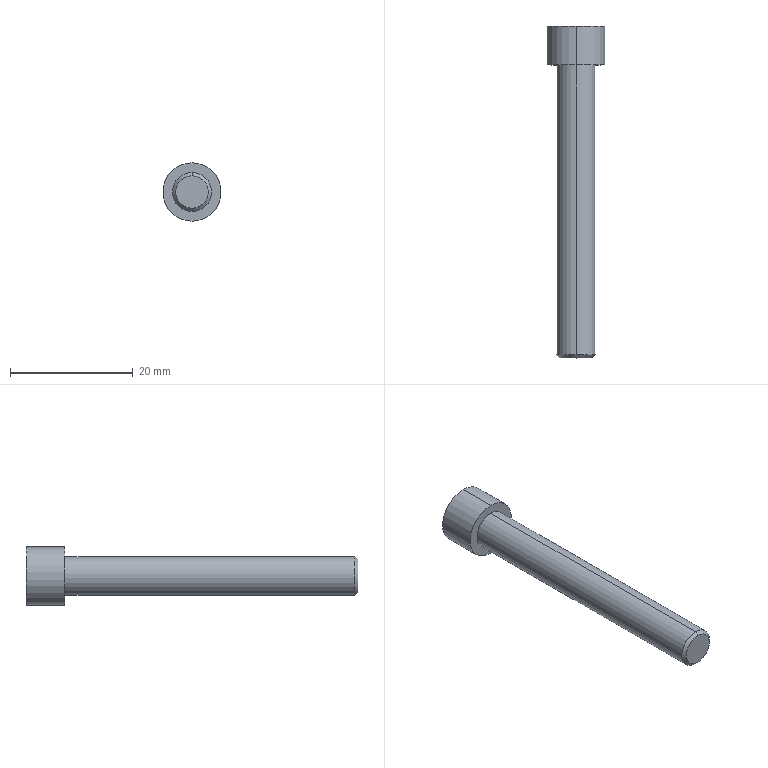Part | STEP file | 4-20.sldasm-Part-206 | 1 solid | 16 faces | box 9.525 x 54.15 x 9.525 mm | volume 1881 mm3 | plane 10 | cylinder 4 | cone 2 | commonest cylinder face diameters 6.35 x2 9.525 x2
STEP:
#1=CARTESIAN_POINT('',(270.795,526.888,-90.641));
#2=VERTEX_POINT('',#1);
#3=CARTESIAN_POINT('',(270.795,526.888,-95.959));
#4=VERTEX_POINT('',#3);
#5=CARTESIAN_POINT('',(270.795,526.888,-93.3));
#6=DIRECTION('',(0.,1.,0.));
#7=DIRECTION('',(0.,0.,1.));
#8=AXIS2_PLACEMENT_3D('',#5,#6,#7);
#9=CIRCLE('',#8,2.659);
#10=EDGE_CURVE('',#2,#4,#9,.T.);
#11=ORIENTED_EDGE('',*,*,#10,.T.);
#12=CARTESIAN_POINT('',(270.795,527.404,-96.475));
#13=VERTEX_POINT('',#12);
#14=CARTESIAN_POINT('',(270.795,527.404,-96.475));
#15=DIRECTION('',(0.,0.7071,-0.7071));
#16=VECTOR('',#15,1000.);
#17=LINE('',#14,#16);
#18=EDGE_CURVE('',#4,#13,#17,.T.);
#19=ORIENTED_EDGE('',*,*,#18,.T.);
#20=CARTESIAN_POINT('',(270.795,527.404,-90.125));
#21=VERTEX_POINT('',#20);
#22=CARTESIAN_POINT('',(270.795,527.404,-93.3));
#23=DIRECTION('',(0.,-1.,0.));
#24=DIRECTION('',(0.,0.,1.));
#25=AXIS2_PLACEMENT_3D('',#22,#23,#24);
#26=CIRCLE('',#25,3.175);
#27=EDGE_CURVE('',#13,#21,#26,.T.);
#28=ORIENTED_EDGE('',*,*,#27,.T.);
#29=CARTESIAN_POINT('',(270.795,527.404,-90.125));
#30=DIRECTION('',(0.,0.7071,0.7071));
#31=VECTOR('',#30,1000.);
#32=LINE('',#29,#31);
#33=EDGE_CURVE('',#2,#21,#32,.T.);
#34=ORIENTED_EDGE('',*,*,#33,.F.);
#35=EDGE_LOOP('',(#11,#19,#28,#34));
#36=FACE_OUTER_BOUND('',#35,.T.);
#37=CARTESIAN_POINT('',(270.795,527.404,-93.3));
#38=DIRECTION('',(0.,1.,0.));
#39=DIRECTION('',(0.,0.,1.));
#40=AXIS2_PLACEMENT_3D('',#37,#38,#39);
#41=CONICAL_SURFACE('',#40,3.175,0.7854);
#42=ADVANCED_FACE('',(#36),#41,.T.);
#43=CARTESIAN_POINT('',(270.795,574.688,-98.063));
#44=VERTEX_POINT('',#43);
#45=CARTESIAN_POINT('',(270.795,574.688,-88.538));
#46=VERTEX_POINT('',#45);
#47=CARTESIAN_POINT('',(270.795,574.688,-93.3));
#48=DIRECTION('',(0.,-1.,0.));
#49=DIRECTION('',(0.,0.,1.));
#50=AXIS2_PLACEMENT_3D('',#47,#48,#49);
#51=CIRCLE('',#50,4.763);
#52=EDGE_CURVE('',#44,#46,#51,.T.);
#53=ORIENTED_EDGE('',*,*,#52,.F.);
#54=CARTESIAN_POINT('',(270.795,581.038,-98.063));
#55=VERTEX_POINT('',#54);
#56=CARTESIAN_POINT('',(270.795,574.688,-98.063));
#57=DIRECTION('',(0.,1.,0.));
#58=VECTOR('',#57,1000.);
#59=LINE('',#56,#58);
#60=EDGE_CURVE('',#44,#55,#59,.T.);
#61=ORIENTED_EDGE('',*,*,#60,.T.);
#62=CARTESIAN_POINT('',(270.795,581.038,-88.538));
#63=VERTEX_POINT('',#62);
#64=CARTESIAN_POINT('',(270.795,581.038,-93.3));
#65=DIRECTION('',(0.,-1.,0.));
#66=DIRECTION('',(0.,0.,1.));
#67=AXIS2_PLACEMENT_3D('',#64,#65,#66);
#68=CIRCLE('',#67,4.763);
#69=EDGE_CURVE('',#55,#63,#68,.T.);
#70=ORIENTED_EDGE('',*,*,#69,.T.);
#71=CARTESIAN_POINT('',(270.795,574.688,-88.538));
#72=DIRECTION('',(0.,1.,0.));
#73=VECTOR('',#72,1000.);
#74=LINE('',#71,#73);
#75=EDGE_CURVE('',#46,#63,#74,.T.);
#76=ORIENTED_EDGE('',*,*,#75,.F.);
#77=EDGE_LOOP('',(#53,#61,#70,#76));
#78=FACE_OUTER_BOUND('',#77,.T.);
#79=CARTESIAN_POINT('',(270.795,574.688,-93.3));
#80=DIRECTION('',(0.,1.,0.));
#81=DIRECTION('',(0.,0.,1.));
#82=AXIS2_PLACEMENT_3D('',#79,#80,#81);
#83=CYLINDRICAL_SURFACE('',#82,4.763);
#84=ADVANCED_FACE('',(#78),#83,.T.);
#85=CARTESIAN_POINT('',(270.795,574.688,-96.475));
#86=VERTEX_POINT('',#85);
#87=CARTESIAN_POINT('',(270.795,574.688,-90.125));
#88=VERTEX_POINT('',#87);
#89=CARTESIAN_POINT('',(270.795,574.688,-93.3));
#90=DIRECTION('',(0.,-1.,0.));
#91=DIRECTION('',(0.,0.,1.));
#92=AXIS2_PLACEMENT_3D('',#89,#90,#91);
#93=CIRCLE('',#92,3.175);
#94=EDGE_CURVE('',#86,#88,#93,.T.);
#95=ORIENTED_EDGE('',*,*,#94,.T.);
#96=CARTESIAN_POINT('',(270.795,574.688,-90.125));
#97=DIRECTION('',(0.,-1.,0.));
#98=VECTOR('',#97,1000.);
#99=LINE('',#96,#98);
#100=EDGE_CURVE('',#88,#21,#99,.T.);
#101=ORIENTED_EDGE('',*,*,#100,.T.);
#102=ORIENTED_EDGE('',*,*,#27,.F.);
#103=CARTESIAN_POINT('',(270.795,574.688,-96.475));
#104=DIRECTION('',(0.,-1.,0.));
#105=VECTOR('',#104,1000.);
#106=LINE('',#103,#105);
#107=EDGE_CURVE('',#86,#13,#106,.T.);
#108=ORIENTED_EDGE('',*,*,#107,.F.);
#109=EDGE_LOOP('',(#95,#101,#102,#108));
#110=FACE_OUTER_BOUND('',#109,.T.);
#111=CARTESIAN_POINT('',(270.795,574.688,-93.3));
#112=DIRECTION('',(0.,-1.,0.));
#113=DIRECTION('',(0.,0.,-1.));
#114=AXIS2_PLACEMENT_3D('',#111,#112,#113);
#115=CYLINDRICAL_SURFACE('',#114,3.175);
#116=ADVANCED_FACE('',(#110),#115,.T.);
#117=ORIENTED_EDGE('',*,*,#100,.F.);
#118=CARTESIAN_POINT('',(270.795,574.688,-93.3));
#119=DIRECTION('',(0.,-1.,0.));
#120=DIRECTION('',(0.,0.,1.));
#121=AXIS2_PLACEMENT_3D('',#118,#119,#120);
#122=CIRCLE('',#121,3.175);
#123=EDGE_CURVE('',#88,#86,#122,.T.);
#124=ORIENTED_EDGE('',*,*,#123,.T.);
#125=ORIENTED_EDGE('',*,*,#107,.T.);
#126=CARTESIAN_POINT('',(270.795,527.404,-93.3));
#127=DIRECTION('',(0.,-1.,0.));
#128=DIRECTION('',(0.,0.,1.));
#129=AXIS2_PLACEMENT_3D('',#126,#127,#128);
#130=CIRCLE('',#129,3.175);
#131=EDGE_CURVE('',#21,#13,#130,.T.);
#132=ORIENTED_EDGE('',*,*,#131,.F.);
#133=EDGE_LOOP('',(#117,#124,#125,#132));
#134=FACE_OUTER_BOUND('',#133,.T.);
#135=CARTESIAN_POINT('',(270.795,574.688,-93.3));
#136=DIRECTION('',(0.,-1.,0.));
#137=DIRECTION('',(0.,0.,-1.));
#138=AXIS2_PLACEMENT_3D('',#135,#136,#137);
#139=CYLINDRICAL_SURFACE('',#138,3.175);
#140=ADVANCED_FACE('',(#134),#139,.T.);
#141=ORIENTED_EDGE('',*,*,#10,.F.);
#142=CARTESIAN_POINT('',(270.795,526.888,-93.3));
#143=DIRECTION('',(0.,1.,0.));
#144=DIRECTION('',(0.,0.,1.));
#145=AXIS2_PLACEMENT_3D('',#142,#143,#144);
#146=CIRCLE('',#145,2.659);
#147=EDGE_CURVE('',#4,#2,#146,.T.);
#148=ORIENTED_EDGE('',*,*,#147,.F.);
#149=EDGE_LOOP('',(#141,#148));
#150=FACE_OUTER_BOUND('',#149,.T.);
#151=CARTESIAN_POINT('',(270.795,526.888,-93.3));
#152=DIRECTION('',(0.,1.,0.));
#153=DIRECTION('',(0.,0.,1.));
#154=AXIS2_PLACEMENT_3D('',#151,#152,#153);
#155=PLANE('',#154);
#156=ADVANCED_FACE('',(#150),#155,.F.);
#157=CARTESIAN_POINT('',(270.795,574.688,-93.3));
#158=DIRECTION('',(0.,-1.,0.));
#159=DIRECTION('',(0.,0.,1.));
#160=AXIS2_PLACEMENT_3D('',#157,#158,#159);
#161=CIRCLE('',#160,4.763);
#162=EDGE_CURVE('',#46,#44,#161,.T.);
#163=ORIENTED_EDGE('',*,*,#162,.T.);
#164=ORIENTED_EDGE('',*,*,#52,.T.);
#165=EDGE_LOOP('',(#163,#164));
#166=FACE_OUTER_BOUND('',#165,.T.);
#167=ORIENTED_EDGE('',*,*,#94,.F.);
#168=ORIENTED_EDGE('',*,*,#123,.F.);
#169=EDGE_LOOP('',(#167,#168));
#170=FACE_BOUND('',#169,.T.);
#171=CARTESIAN_POINT('',(270.795,574.688,-93.3));
#172=DIRECTION('',(0.,-1.,0.));
#173=DIRECTION('',(0.,0.,-1.));
#174=AXIS2_PLACEMENT_3D('',#171,#172,#173);
#175=PLANE('',#174);
#176=ADVANCED_FACE('',(#166,#170),#175,.T.);
#177=CARTESIAN_POINT('',(273.176,581.038,-94.675));
#178=VERTEX_POINT('',#177);
#179=CARTESIAN_POINT('',(273.176,581.038,-91.925));
#180=VERTEX_POINT('',#179);
#181=CARTESIAN_POINT('',(273.176,581.038,-94.675));
#182=DIRECTION('',(0.,0.,1.));
#183=VECTOR('',#182,1000.);
#184=LINE('',#181,#183);
#185=EDGE_CURVE('',#178,#180,#184,.T.);
#186=ORIENTED_EDGE('',*,*,#185,.T.);
#187=CARTESIAN_POINT('',(270.795,581.038,-90.55));
#188=VERTEX_POINT('',#187);
#189=CARTESIAN_POINT('',(273.176,581.038,-91.925));
#190=DIRECTION('',(-0.866,0.,0.5));
#191=VECTOR('',#190,1000.);
#192=LINE('',#189,#191);
#193=EDGE_CURVE('',#180,#188,#192,.T.);
#194=ORIENTED_EDGE('',*,*,#193,.T.);
#195=CARTESIAN_POINT('',(268.414,581.038,-91.925));
#196=VERTEX_POINT('',#195);
#197=CARTESIAN_POINT('',(270.795,581.038,-90.55));
#198=DIRECTION('',(-0.866,0.,-0.5));
#199=VECTOR('',#198,1000.);
#200=LINE('',#197,#199);
#201=EDGE_CURVE('',#188,#196,#200,.T.);
#202=ORIENTED_EDGE('',*,*,#201,.T.);
#203=CARTESIAN_POINT('',(268.414,581.038,-94.675));
#204=VERTEX_POINT('',#203);
#205=CARTESIAN_POINT('',(268.414,581.038,-91.925));
#206=DIRECTION('',(0.,0.,-1.));
#207=VECTOR('',#206,1000.);
#208=LINE('',#205,#207);
#209=EDGE_CURVE('',#196,#204,#208,.T.);
#210=ORIENTED_EDGE('',*,*,#209,.T.);
#211=CARTESIAN_POINT('',(270.795,581.038,-96.05));
#212=VERTEX_POINT('',#211);
#213=CARTESIAN_POINT('',(268.414,581.038,-94.675));
#214=DIRECTION('',(0.866,0.,-0.5));
#215=VECTOR('',#214,1000.);
#216=LINE('',#213,#215);
#217=EDGE_CURVE('',#204,#212,#216,.T.);
#218=ORIENTED_EDGE('',*,*,#217,.T.);
#219=CARTESIAN_POINT('',(270.795,581.038,-96.05));
#220=DIRECTION('',(0.866,0.,0.5));
#221=VECTOR('',#220,1000.);
#222=LINE('',#219,#221);
#223=EDGE_CURVE('',#212,#178,#222,.T.);
#224=ORIENTED_EDGE('',*,*,#223,.T.);
#225=EDGE_LOOP('',(#186,#194,#202,#210,#218,#224));
#226=FACE_BOUND('',#225,.T.);
#227=CARTESIAN_POINT('',(270.795,581.038,-93.3));
#228=DIRECTION('',(0.,-1.,0.));
#229=DIRECTION('',(0.,0.,1.));
#230=AXIS2_PLACEMENT_3D('',#227,#228,#229);
#231=CIRCLE('',#230,4.763);
#232=EDGE_CURVE('',#63,#55,#231,.T.);
#233=ORIENTED_EDGE('',*,*,#232,.F.);
#234=ORIENTED_EDGE('',*,*,#69,.F.);
#235=EDGE_LOOP('',(#233,#234));
#236=FACE_OUTER_BOUND('',#235,.T.);
#237=CARTESIAN_POINT('',(270.795,581.038,-93.3));
#238=DIRECTION('',(0.,1.,0.));
#239=DIRECTION('',(0.,0.,1.));
#240=AXIS2_PLACEMENT_3D('',#237,#238,#239);
#241=PLANE('',#240);
#242=ADVANCED_FACE('',(#226,#236),#241,.T.);
#243=ORIENTED_EDGE('',*,*,#60,.F.);
#244=ORIENTED_EDGE('',*,*,#162,.F.);
#245=ORIENTED_EDGE('',*,*,#75,.T.);
#246=ORIENTED_EDGE('',*,*,#232,.T.);
#247=EDGE_LOOP('',(#243,#244,#245,#246));
#248=FACE_OUTER_BOUND('',#247,.T.);
#249=CARTESIAN_POINT('',(270.795,574.688,-93.3));
#250=DIRECTION('',(0.,1.,0.));
#251=DIRECTION('',(0.,0.,1.));
#252=AXIS2_PLACEMENT_3D('',#249,#250,#251);
#253=CYLINDRICAL_SURFACE('',#252,4.763);
#254=ADVANCED_FACE('',(#248),#253,.T.);
#255=ORIENTED_EDGE('',*,*,#18,.F.);
#256=ORIENTED_EDGE('',*,*,#147,.T.);
#257=ORIENTED_EDGE('',*,*,#33,.T.);
#258=ORIENTED_EDGE('',*,*,#131,.T.);
#259=EDGE_LOOP('',(#255,#256,#257,#258));
#260=FACE_OUTER_BOUND('',#259,.T.);
#261=CARTESIAN_POINT('',(270.795,527.404,-93.3));
#262=DIRECTION('',(0.,1.,0.));
#263=DIRECTION('',(0.,0.,1.));
#264=AXIS2_PLACEMENT_3D('',#261,#262,#263);
#265=CONICAL_SURFACE('',#264,3.175,0.7854);
#266=ADVANCED_FACE('',(#260),#265,.T.);
#267=ORIENTED_EDGE('',*,*,#185,.F.);
#268=CARTESIAN_POINT('',(273.176,576.847,-94.675));
#269=VERTEX_POINT('',#268);
#270=CARTESIAN_POINT('',(273.176,576.847,-94.675));
#271=DIRECTION('',(0.,1.,0.));
#272=VECTOR('',#271,1000.);
#273=LINE('',#270,#272);
#274=EDGE_CURVE('',#269,#178,#273,.T.);
#275=ORIENTED_EDGE('',*,*,#274,.F.);
#276=CARTESIAN_POINT('',(273.176,576.847,-91.925));
#277=VERTEX_POINT('',#276);
#278=CARTESIAN_POINT('',(273.176,576.847,-94.675));
#279=DIRECTION('',(0.,0.,1.));
#280=VECTOR('',#279,1000.);
#281=LINE('',#278,#280);
#282=EDGE_CURVE('',#269,#277,#281,.T.);
#283=ORIENTED_EDGE('',*,*,#282,.T.);
#284=CARTESIAN_POINT('',(273.176,576.847,-91.925));
#285=DIRECTION('',(0.,1.,0.));
#286=VECTOR('',#285,1000.);
#287=LINE('',#284,#286);
#288=EDGE_CURVE('',#277,#180,#287,.T.);
#289=ORIENTED_EDGE('',*,*,#288,.T.);
#290=EDGE_LOOP('',(#267,#275,#283,#289));
#291=FACE_OUTER_BOUND('',#290,.T.);
#292=CARTESIAN_POINT('',(273.176,576.847,-94.675));
#293=DIRECTION('',(1.,0.,0.));
#294=DIRECTION('',(0.,-1.,0.));
#295=AXIS2_PLACEMENT_3D('',#292,#293,#294);
#296=PLANE('',#295);
#297=ADVANCED_FACE('',(#291),#296,.F.);
#298=ORIENTED_EDGE('',*,*,#193,.F.);
#299=ORIENTED_EDGE('',*,*,#288,.F.);
#300=CARTESIAN_POINT('',(270.795,576.847,-90.55));
#301=VERTEX_POINT('',#300);
#302=CARTESIAN_POINT('',(273.176,576.847,-91.925));
#303=DIRECTION('',(-0.866,0.,0.5));
#304=VECTOR('',#303,1000.);
#305=LINE('',#302,#304);
#306=EDGE_CURVE('',#277,#301,#305,.T.);
#307=ORIENTED_EDGE('',*,*,#306,.T.);
#308=CARTESIAN_POINT('',(270.795,576.847,-90.55));
#309=DIRECTION('',(0.,1.,0.));
#310=VECTOR('',#309,1000.);
#311=LINE('',#308,#310);
#312=EDGE_CURVE('',#301,#188,#311,.T.);
#313=ORIENTED_EDGE('',*,*,#312,.T.);
#314=EDGE_LOOP('',(#298,#299,#307,#313));
#315=FACE_OUTER_BOUND('',#314,.T.);
#316=CARTESIAN_POINT('',(273.176,576.847,-91.925));
#317=DIRECTION('',(0.5,0.,0.866));
#318=DIRECTION('',(-0.866,0.,0.5));
#319=AXIS2_PLACEMENT_3D('',#316,#317,#318);
#320=PLANE('',#319);
#321=ADVANCED_FACE('',(#315),#320,.F.);
#322=ORIENTED_EDGE('',*,*,#201,.F.);
#323=ORIENTED_EDGE('',*,*,#312,.F.);
#324=CARTESIAN_POINT('',(268.414,576.847,-91.925));
#325=VERTEX_POINT('',#324);
#326=CARTESIAN_POINT('',(270.795,576.847,-90.55));
#327=DIRECTION('',(-0.866,0.,-0.5));
#328=VECTOR('',#327,1000.);
#329=LINE('',#326,#328);
#330=EDGE_CURVE('',#301,#325,#329,.T.);
#331=ORIENTED_EDGE('',*,*,#330,.T.);
#332=CARTESIAN_POINT('',(268.414,576.847,-91.925));
#333=DIRECTION('',(0.,1.,0.));
#334=VECTOR('',#333,1000.);
#335=LINE('',#332,#334);
#336=EDGE_CURVE('',#325,#196,#335,.T.);
#337=ORIENTED_EDGE('',*,*,#336,.T.);
#338=EDGE_LOOP('',(#322,#323,#331,#337));
#339=FACE_OUTER_BOUND('',#338,.T.);
#340=CARTESIAN_POINT('',(270.795,576.847,-90.55));
#341=DIRECTION('',(-0.5,0.,0.866));
#342=DIRECTION('',(-0.866,0.,-0.5));
#343=AXIS2_PLACEMENT_3D('',#340,#341,#342);
#344=PLANE('',#343);
#345=ADVANCED_FACE('',(#339),#344,.F.);
#346=ORIENTED_EDGE('',*,*,#209,.F.);
#347=ORIENTED_EDGE('',*,*,#336,.F.);
#348=CARTESIAN_POINT('',(268.414,576.847,-94.675));
#349=VERTEX_POINT('',#348);
#350=CARTESIAN_POINT('',(268.414,576.847,-91.925));
#351=DIRECTION('',(0.,0.,-1.));
#352=VECTOR('',#351,1000.);
#353=LINE('',#350,#352);
#354=EDGE_CURVE('',#325,#349,#353,.T.);
#355=ORIENTED_EDGE('',*,*,#354,.T.);
#356=CARTESIAN_POINT('',(268.414,576.847,-94.675));
#357=DIRECTION('',(0.,1.,0.));
#358=VECTOR('',#357,1000.);
#359=LINE('',#356,#358);
#360=EDGE_CURVE('',#349,#204,#359,.T.);
#361=ORIENTED_EDGE('',*,*,#360,.T.);
#362=EDGE_LOOP('',(#346,#347,#355,#361));
#363=FACE_OUTER_BOUND('',#362,.T.);
#364=CARTESIAN_POINT('',(268.414,576.847,-91.925));
#365=DIRECTION('',(-1.,0.,0.));
#366=DIRECTION('',(0.,1.,0.));
#367=AXIS2_PLACEMENT_3D('',#364,#365,#366);
#368=PLANE('',#367);
#369=ADVANCED_FACE('',(#363),#368,.F.);
#370=ORIENTED_EDGE('',*,*,#217,.F.);
#371=ORIENTED_EDGE('',*,*,#360,.F.);
#372=CARTESIAN_POINT('',(270.795,576.847,-96.05));
#373=VERTEX_POINT('',#372);
#374=CARTESIAN_POINT('',(268.414,576.847,-94.675));
#375=DIRECTION('',(0.866,0.,-0.5));
#376=VECTOR('',#375,1000.);
#377=LINE('',#374,#376);
#378=EDGE_CURVE('',#349,#373,#377,.T.);
#379=ORIENTED_EDGE('',*,*,#378,.T.);
#380=CARTESIAN_POINT('',(270.795,576.847,-96.05));
#381=DIRECTION('',(0.,1.,0.));
#382=VECTOR('',#381,1000.);
#383=LINE('',#380,#382);
#384=EDGE_CURVE('',#373,#212,#383,.T.);
#385=ORIENTED_EDGE('',*,*,#384,.T.);
#386=EDGE_LOOP('',(#370,#371,#379,#385));
#387=FACE_OUTER_BOUND('',#386,.T.);
#388=CARTESIAN_POINT('',(268.414,576.847,-94.675));
#389=DIRECTION('',(-0.5,0.,-0.866));
#390=DIRECTION('',(0.866,0.,-0.5));
#391=AXIS2_PLACEMENT_3D('',#388,#389,#390);
#392=PLANE('',#391);
#393=ADVANCED_FACE('',(#387),#392,.F.);
#394=ORIENTED_EDGE('',*,*,#223,.F.);
#395=ORIENTED_EDGE('',*,*,#384,.F.);
#396=CARTESIAN_POINT('',(270.795,576.847,-96.05));
#397=DIRECTION('',(0.866,0.,0.5));
#398=VECTOR('',#397,1000.);
#399=LINE('',#396,#398);
#400=EDGE_CURVE('',#373,#269,#399,.T.);
#401=ORIENTED_EDGE('',*,*,#400,.T.);
#402=ORIENTED_EDGE('',*,*,#274,.T.);
#403=EDGE_LOOP('',(#394,#395,#401,#402));
#404=FACE_OUTER_BOUND('',#403,.T.);
#405=CARTESIAN_POINT('',(270.795,576.847,-96.05));
#406=DIRECTION('',(0.5,0.,-0.866));
#407=DIRECTION('',(0.866,0.,0.5));
#408=AXIS2_PLACEMENT_3D('',#405,#406,#407);
#409=PLANE('',#408);
#410=ADVANCED_FACE('',(#404),#409,.F.);
#411=ORIENTED_EDGE('',*,*,#282,.F.);
#412=ORIENTED_EDGE('',*,*,#400,.F.);
#413=ORIENTED_EDGE('',*,*,#378,.F.);
#414=ORIENTED_EDGE('',*,*,#354,.F.);
#415=ORIENTED_EDGE('',*,*,#330,.F.);
#416=ORIENTED_EDGE('',*,*,#306,.F.);
#417=EDGE_LOOP('',(#411,#412,#413,#414,#415,#416));
#418=FACE_OUTER_BOUND('',#417,.T.);
#419=CARTESIAN_POINT('',(273.176,576.847,-91.925));
#420=DIRECTION('',(0.,1.,0.));
#421=DIRECTION('',(0.,0.,1.));
#422=AXIS2_PLACEMENT_3D('',#419,#420,#421);
#423=PLANE('',#422);
#424=ADVANCED_FACE('',(#418),#423,.T.);
#425=CLOSED_SHELL('',(#42,#84,#116,#140,#156,#176,#242,#254,#266,#297,#321,#345,#369,#393,#410,#424));
#426=MANIFOLD_SOLID_BREP('',#425);
#427=CARTESIAN_POINT('',(0.,0.,0.));
#428=DIRECTION('',(0.,0.,1.));
#429=DIRECTION('',(1.,0.,0.));
#430=AXIS2_PLACEMENT_3D('',#427,#428,#429);
#431=(LENGTH_UNIT()NAMED_UNIT(*)SI_UNIT(.MILLI.,.METRE.));
#432=UNCERTAINTY_MEASURE_WITH_UNIT(LENGTH_MEASURE(0.00001),#431,'','');
#433=(NAMED_UNIT(*)PLANE_ANGLE_UNIT()SI_UNIT($,.RADIAN.));
#434=(NAMED_UNIT(*)SI_UNIT($,.STERADIAN.)SOLID_ANGLE_UNIT());
#435=(GEOMETRIC_REPRESENTATION_CONTEXT(3)GLOBAL_UNCERTAINTY_ASSIGNED_CONTEXT((#432))GLOBAL_UNIT_ASSIGNED_CONTEXT((#431,#433,#434))REPRESENTATION_CONTEXT('',''));
#436=ADVANCED_BREP_SHAPE_REPRESENTATION('',(#426,#430),#435);